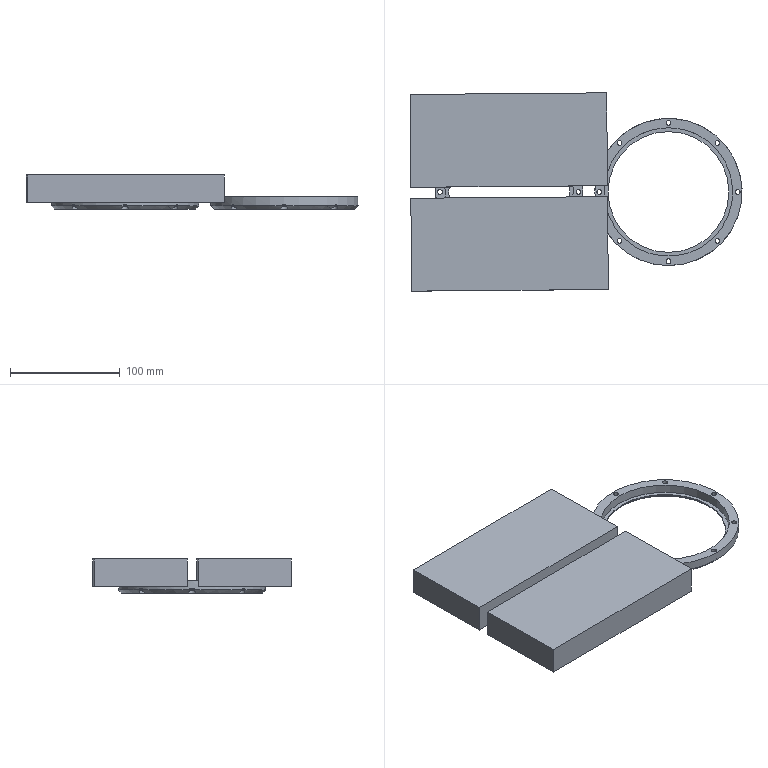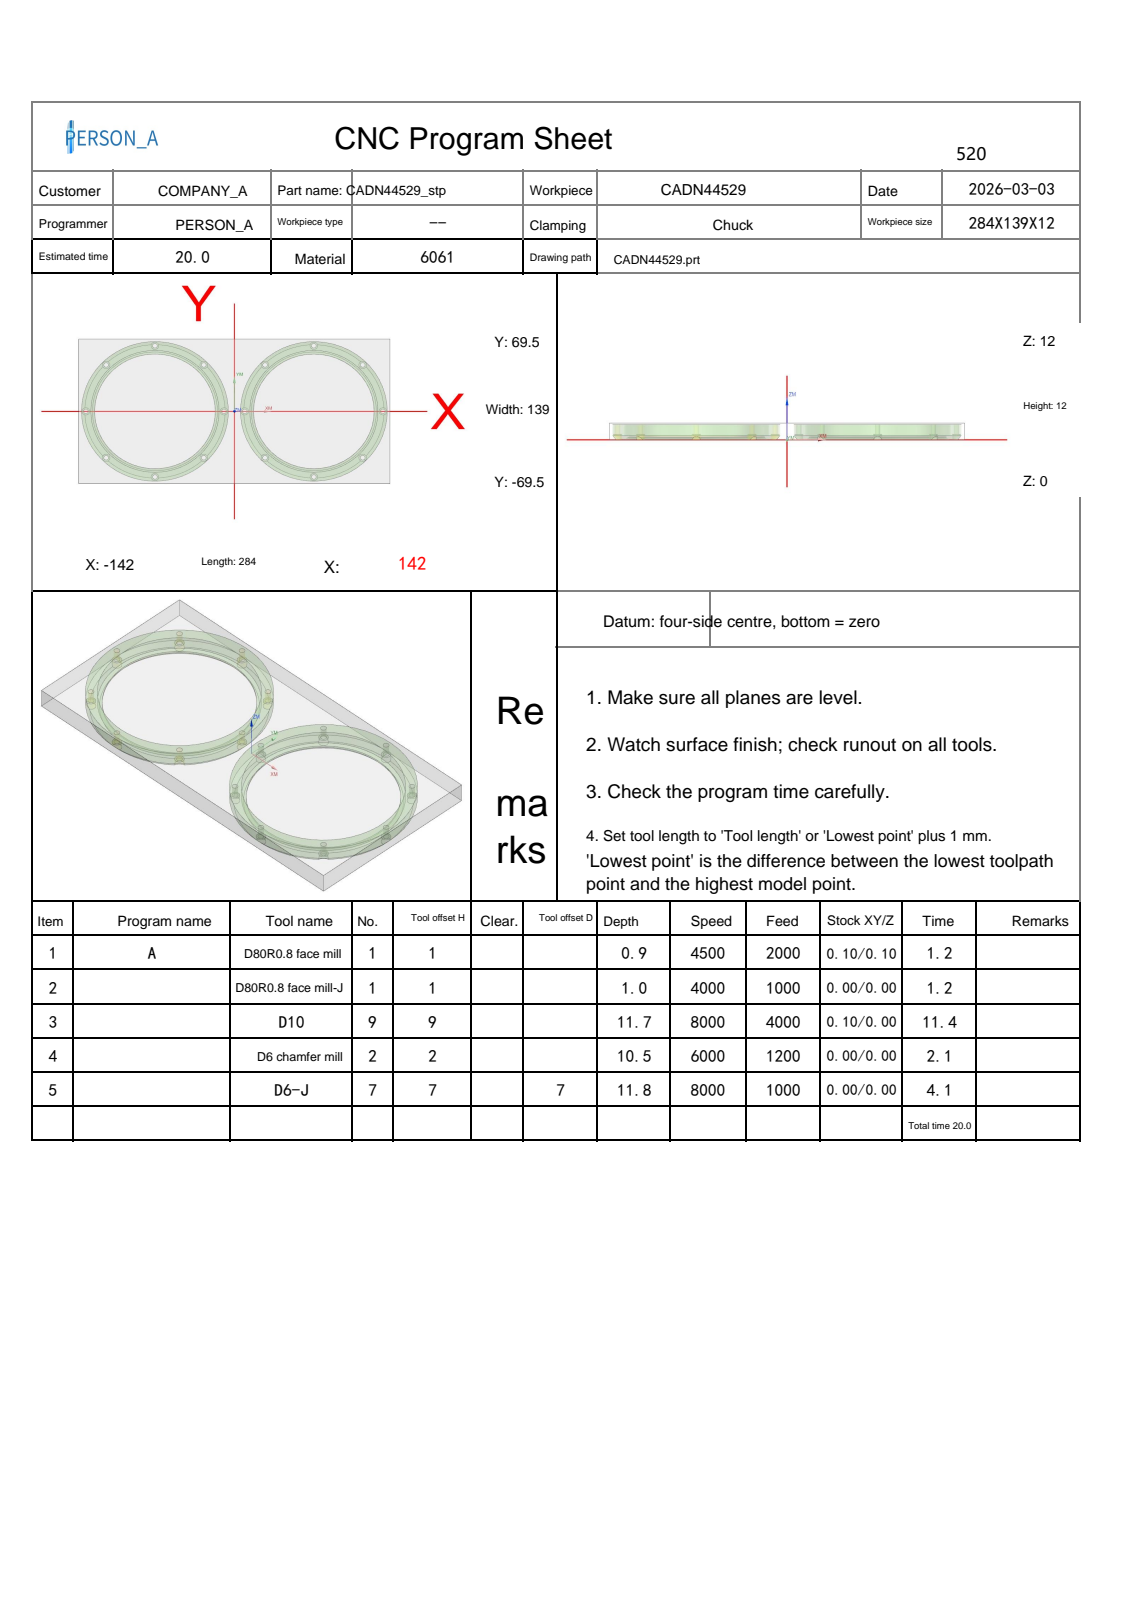NC program | NX | posted by the shop | part box 302.234 x 180.468 x 31 mm
Whole program:
%
O0001
(Machine time: 20.83 MIN)
(===Total Tool:4===)
(T1=D80R0.8 face mill D=80.  R=0.8  D-  H01 Z=11.   )
(T9=D10     D=10.  R=0.   D-  H09 Z=0.3   )
(T2=D6 chamfer mill   D=6.   R=0.   D-  H02 Z=1.5   )
(T7=D6-J    D=6.   R=0.   D7  H07 Z=0.2   )
G80 G90 G17 G49 G40
G91 G28 Z0
M01
N1 T01 M06
(D80R0.8 face mill  D=80. R=0.8 H=01 ce=0.10 di=0.10)
G00 G90 G54 X-183.526 Y43.097 M03 S4500
G43 H01 Z61.
M08
Z13.55
G01 Z11.55 F2000.
X-170.543
X165.174
G02 X172.655 Y37.93 I0.0 J-8.
X178.96 Y11.664 I-100.155 J-37.93
X179.003 Y10.88 I-7.157 J-.784
X171.803 Y3.68 I-7.2 J0.0
G01 X-172.338
G03 X-179.535 Y-3.52 I.004 J-7.2
X-179.531 Y-3.77 I7.2 J0.0
X-175.316 Y-29.976 I107.031 J3.77
X-167.636 Y-35.737 I7.68 J2.239
G01 X173.459
X186.109
Z13.55
G00 X-183.526 Y43.097
Z13.1
G01 Z11.1
X-170.543
X165.174
G02 X172.655 Y37.93 I0.0 J-8.
X178.96 Y11.664 I-100.155 J-37.93
X179.003 Y10.88 I-7.157 J-.784
X171.803 Y3.68 I-7.2 J0.0
G01 X-172.338
G03 X-179.535 Y-3.52 I.004 J-7.2
X-179.531 Y-3.77 I7.2 J0.0
X-175.316 Y-29.976 I107.031 J3.77
X-167.636 Y-35.737 I7.68 J2.239
G01 X173.459
X186.109
Z13.1
G00 Z61.
G91 G28 Z0.0
M05
M09
G91 G28 Z0.0
M01
N2 T01 M06
(D80R0.8 face mill-J  D=80. R=0.8 H=01 ce=0.00 di=0.00)
G00 G90 G54 X-183.459 Y42.999 M03 S4000
G43 H01 Z61.
M08
Z13.
G01 Z11. F1000.
X-170.479
X165.106
G02 X172.589 Y37.827 I0.0 J-8.
X178.861 Y11.665 I-100.089 J-37.827
X178.904 Y10.88 I-7.157 J-.785
X171.704 Y3.68 I-7.2 J0.0
G01 X-172.24
G03 X-179.437 Y-3.52 I.004 J-7.2
X-179.433 Y-3.77 I7.2 J0.0
X-175.244 Y-29.872 I106.933 J3.77
X-167.563 Y-35.639 I7.682 J2.233
G01 X173.389
X186.037
Z13.
G00 Z61.
G91 G28 Z0.0
M05
M09
G91 G28 Z0.0
M01
N3 T09 M06
(D10  D=10. R=0. H=09 ce=0.10 di=0.10)
G00 G90 G54 X-118.783 Y18.61 M03 S8000
G43 H09 Z61.
M08
Z13.
G01 X-119.955 Y15.526 Z12.827 F4000.
X-121.201 Y11.011 Z12.581
X-122.018 Y6.399 Z12.336
X-122.4 Y1.731 Z12.09
Y0.0 Z12.
G03 X-72.5 Y-49.9 Z11.854 I49.9 J0.0
X-22.6 Y0.0 Z11.707 I0.0 J49.9
X-72.5 Y49.9 Z11.561 I-49.9 J0.0
X-122.4 Y0.0 Z11.415 I0.0 J-49.9
X-72.5 Y-49.9 Z11.269 I49.9 J0.0
X-22.6 Y0.0 Z11.122 I0.0 J49.9
X-72.5 Y49.9 Z10.976 I-49.9 J0.0
X-122.4 Y0.0 Z10.83 I0.0 J-49.9
X-72.5 Y-49.9 Z10.684 I49.9 J0.0
X-22.6 Y0.0 Z10.537 I0.0 J49.9
X-72.5 Y49.9 Z10.391 I-49.9 J0.0
X-122.4 Y0.0 Z10.245 I0.0 J-49.9
X-72.5 Y-49.9 Z10.099 I49.9 J0.0
X-22.6 Y0.0 Z9.952 I0.0 J49.9
X-72.5 Y49.9 Z9.806 I-49.9 J0.0
X-122.4 Y0.0 Z9.66 I0.0 J-49.9
X-72.5 Y-49.9 Z9.514 I49.9 J0.0
X-22.6 Y0.0 Z9.367 I0.0 J49.9
X-72.5 Y49.9 Z9.221 I-49.9 J0.0
X-122.4 Y0.0 Z9.075 I0.0 J-49.9
X-72.5 Y-49.9 Z8.929 I49.9 J0.0
X-22.6 Y0.0 Z8.782 I0.0 J49.9
X-72.5 Y49.9 Z8.636 I-49.9 J0.0
X-122.4 Y0.0 Z8.49 I0.0 J-49.9
X-72.5 Y-49.9 Z8.344 I49.9 J0.0
X-22.6 Y0.0 Z8.197 I0.0 J49.9
X-72.5 Y49.9 Z8.051 I-49.9 J0.0
X-122.4 Y0.0 Z7.905 I0.0 J-49.9
X-72.5 Y-49.9 Z7.759 I49.9 J0.0
X-22.6 Y0.0 Z7.612 I0.0 J49.9
X-72.5 Y49.9 Z7.466 I-49.9 J0.0
X-122.4 Y0.0 Z7.32 I0.0 J-49.9
X-72.5 Y-49.9 Z7.174 I49.9 J0.0
X-22.6 Y0.0 Z7.027 I0.0 J49.9
X-72.5 Y49.9 Z6.881 I-49.9 J0.0
X-122.4 Y0.0 Z6.735 I0.0 J-49.9
X-72.5 Y-49.9 Z6.589 I49.9 J0.0
X-22.6 Y0.0 Z6.442 I0.0 J49.9
X-72.5 Y49.9 Z6.296 I-49.9 J0.0
X-122.4 Y0.0 Z6.15 I0.0 J-49.9
X-72.5 Y-49.9 Z6.004 I49.9 J0.0
X-22.6 Y0.0 Z5.857 I0.0 J49.9
X-72.5 Y49.9 Z5.711 I-49.9 J0.0
X-122.4 Y0.0 Z5.565 I0.0 J-49.9
X-72.5 Y-49.9 Z5.419 I49.9 J0.0
X-22.6 Y0.0 Z5.272 I0.0 J49.9
X-72.5 Y49.9 Z5.126 I-49.9 J0.0
X-122.4 Y0.0 Z4.98 I0.0 J-49.9
X-72.5 Y-49.9 Z4.834 I49.9 J0.0
X-22.6 Y0.0 Z4.687 I0.0 J49.9
X-72.5 Y49.9 Z4.541 I-49.9 J0.0
X-122.4 Y0.0 Z4.395 I0.0 J-49.9
X-72.5 Y-49.9 Z4.249 I49.9 J0.0
X-22.6 Y0.0 Z4.103 I0.0 J49.9
X-72.5 Y49.9 Z3.956 I-49.9 J0.0
X-122.4 Y0.0 Z3.81 I0.0 J-49.9
X-72.5 Y-49.9 Z3.664 I49.9 J0.0
X-22.6 Y0.0 Z3.518 I0.0 J49.9
X-72.5 Y49.9 Z3.371 I-49.9 J0.0
X-122.4 Y0.0 Z3.225 I0.0 J-49.9
X-72.5 Y-49.9 Z3.079 I49.9 J0.0
X-22.6 Y0.0 Z2.933 I0.0 J49.9
X-72.5 Y49.9 Z2.786 I-49.9 J0.0
X-122.4 Y0.0 Z2.64 I0.0 J-49.9
X-72.5 Y-49.9 Z2.494 I49.9 J0.0
X-22.6 Y0.0 Z2.348 I0.0 J49.9
X-72.5 Y49.9 Z2.201 I-49.9 J0.0
X-122.4 Y0.0 Z2.055 I0.0 J-49.9
X-72.5 Y-49.9 Z1.909 I49.9 J0.0
X-22.6 Y0.0 Z1.763 I0.0 J49.9
X-72.5 Y49.9 Z1.616 I-49.9 J0.0
X-122.4 Y0.0 Z1.47 I0.0 J-49.9
X-72.5 Y-49.9 Z1.324 I49.9 J0.0
X-22.6 Y0.0 Z1.178 I0.0 J49.9
X-72.5 Y49.9 Z1.031 I-49.9 J0.0
X-122.4 Y0.0 Z.885 I0.0 J-49.9
X-72.5 Y-49.9 Z.739 I49.9 J0.0
X-22.6 Y0.0 Z.593 I0.0 J49.9
X-72.5 Y49.9 Z.446 I-49.9 J0.0
X-122.4 Y0.0 Z.3 I0.0 J-49.9
X-72.5 Y-49.9 I49.9 J0.0
X-22.6 Y0.0 I0.0 J49.9
X-72.5 Y49.9 I-49.9 J0.0
X-122.4 Y0.0 I0.0 J-49.9
X-122.398 Y-.4 I49.9 J0.0
G01 Z1.3
G00 Z61.
X53.89 Y-46.283
Z13.
G01 X56.974 Y-47.455 Z12.827
X61.489 Y-48.701 Z12.581
X66.101 Y-49.518 Z12.336
X70.769 Y-49.9 Z12.09
X72.5 Z12.
G03 X122.4 Y0.0 Z11.854 I0.0 J49.9
X72.5 Y49.9 Z11.707 I-49.9 J0.0
X22.6 Y0.0 Z11.561 I0.0 J-49.9
X72.5 Y-49.9 Z11.415 I49.9 J0.0
X122.4 Y0.0 Z11.269 I0.0 J49.9
X72.5 Y49.9 Z11.122 I-49.9 J0.0
X22.6 Y0.0 Z10.976 I0.0 J-49.9
X72.5 Y-49.9 Z10.83 I49.9 J0.0
X122.4 Y0.0 Z10.684 I0.0 J49.9
X72.5 Y49.9 Z10.537 I-49.9 J0.0
X22.6 Y0.0 Z10.391 I0.0 J-49.9
X72.5 Y-49.9 Z10.245 I49.9 J0.0
X122.4 Y0.0 Z10.099 I0.0 J49.9
X72.5 Y49.9 Z9.952 I-49.9 J0.0
X22.6 Y0.0 Z9.806 I0.0 J-49.9
X72.5 Y-49.9 Z9.66 I49.9 J0.0
X122.4 Y0.0 Z9.514 I0.0 J49.9
X72.5 Y49.9 Z9.367 I-49.9 J0.0
X22.6 Y0.0 Z9.221 I0.0 J-49.9
X72.5 Y-49.9 Z9.075 I49.9 J0.0
X122.4 Y0.0 Z8.929 I0.0 J49.9
X72.5 Y49.9 Z8.782 I-49.9 J0.0
X22.6 Y0.0 Z8.636 I0.0 J-49.9
X72.5 Y-49.9 Z8.49 I49.9 J0.0
X122.4 Y0.0 Z8.344 I0.0 J49.9
X72.5 Y49.9 Z8.197 I-49.9 J0.0
X22.6 Y0.0 Z8.051 I0.0 J-49.9
X72.5 Y-49.9 Z7.905 I49.9 J0.0
X122.4 Y0.0 Z7.759 I0.0 J49.9
X72.5 Y49.9 Z7.612 I-49.9 J0.0
X22.6 Y0.0 Z7.466 I0.0 J-49.9
X72.5 Y-49.9 Z7.32 I49.9 J0.0
X122.4 Y0.0 Z7.174 I0.0 J49.9
X72.5 Y49.9 Z7.027 I-49.9 J0.0
X22.6 Y0.0 Z6.881 I0.0 J-49.9
X72.5 Y-49.9 Z6.735 I49.9 J0.0
X122.4 Y0.0 Z6.589 I0.0 J49.9
X72.5 Y49.9 Z6.442 I-49.9 J0.0
X22.6 Y0.0 Z6.296 I0.0 J-49.9
X72.5 Y-49.9 Z6.15 I49.9 J0.0
X122.4 Y0.0 Z6.004 I0.0 J49.9
X72.5 Y49.9 Z5.857 I-49.9 J0.0
X22.6 Y0.0 Z5.711 I0.0 J-49.9
X72.5 Y-49.9 Z5.565 I49.9 J0.0
X122.4 Y0.0 Z5.419 I0.0 J49.9
X72.5 Y49.9 Z5.272 I-49.9 J0.0
X22.6 Y0.0 Z5.126 I0.0 J-49.9
X72.5 Y-49.9 Z4.98 I49.9 J0.0
X122.4 Y0.0 Z4.834 I0.0 J49.9
X72.5 Y49.9 Z4.687 I-49.9 J0.0
X22.6 Y0.0 Z4.541 I0.0 J-49.9
X72.5 Y-49.9 Z4.395 I49.9 J0.0
X122.4 Y0.0 Z4.249 I0.0 J49.9
X72.5 Y49.9 Z4.103 I-49.9 J0.0
X22.6 Y0.0 Z3.956 I0.0 J-49.9
X72.5 Y-49.9 Z3.81 I49.9 J0.0
X122.4 Y0.0 Z3.664 I0.0 J49.9
X72.5 Y49.9 Z3.518 I-49.9 J0.0
X22.6 Y0.0 Z3.371 I0.0 J-49.9
X72.5 Y-49.9 Z3.225 I49.9 J0.0
X122.4 Y0.0 Z3.079 I0.0 J49.9
X72.5 Y49.9 Z2.933 I-49.9 J0.0
X22.6 Y0.0 Z2.786 I0.0 J-49.9
X72.5 Y-49.9 Z2.64 I49.9 J0.0
X122.4 Y0.0 Z2.494 I0.0 J49.9
X72.5 Y49.9 Z2.348 I-49.9 J0.0
X22.6 Y0.0 Z2.201 I0.0 J-49.9
X72.5 Y-49.9 Z2.055 I49.9 J0.0
X122.4 Y0.0 Z1.909 I0.0 J49.9
X72.5 Y49.9 Z1.763 I-49.9 J0.0
X22.6 Y0.0 Z1.616 I0.0 J-49.9
X72.5 Y-49.9 Z1.47 I49.9 J0.0
X122.4 Y0.0 Z1.324 I0.0 J49.9
X72.5 Y49.9 Z1.178 I-49.9 J0.0
X22.6 Y0.0 Z1.031 I0.0 J-49.9
X72.5 Y-49.9 Z.885 I49.9 J0.0
X122.4 Y0.0 Z.739 I0.0 J49.9
X72.5 Y49.9 Z.593 I-49.9 J0.0
X22.6 Y0.0 Z.446 I0.0 J-49.9
X72.5 Y-49.9 Z.3 I49.9 J0.0
X122.4 Y0.0 I0.0 J49.9
X72.5 Y49.9 I-49.9 J0.0
X22.6 Y0.0 I0.0 J-49.9
X72.5 Y-49.9 I49.9 J0.0
X72.9 Y-49.898 I0.0 J49.9
G01 Z1.3
G00 Z61.
G00 G90 X-91.164 Y-50.002 M03 S8000
Z61.
Z12.
G01 X-89.077 Y-50.793 Z11.883 F4000.
X-84.237 Y-52.125 Z11.62
X-79.294 Y-52.996 Z11.357
X-74.29 Y-53.4 Z11.094
X-72.5 Z11.
G03 X-19.1 Y0.0 Z10.859 I0.0 J53.4
X-72.5 Y53.4 Z10.718 I-53.4 J0.0
X-125.9 Y0.0 Z10.577 I0.0 J-53.4
X-72.5 Y-53.4 Z10.436 I53.4 J0.0
X-19.1 Y0.0 Z10.295 I0.0 J53.4
X-72.5 Y53.4 Z10.154 I-53.4 J0.0
X-125.9 Y0.0 Z10.013 I0.0 J-53.4
X-72.5 Y-53.4 Z9.872 I53.4 J0.0
X-19.1 Y0.0 Z9.73 I0.0 J53.4
X-72.5 Y53.4 Z9.589 I-53.4 J0.0
X-125.9 Y0.0 Z9.448 I0.0 J-53.4
X-72.5 Y-53.4 Z9.307 I53.4 J0.0
X-19.1 Y0.0 Z9.166 I0.0 J53.4
X-72.5 Y53.4 Z9.025 I-53.4 J0.0
X-125.9 Y0.0 Z8.884 I0.0 J-53.4
X-72.5 Y-53.4 Z8.743 I53.4 J0.0
X-19.1 Y0.0 Z8.602 I0.0 J53.4
X-72.5 Y53.4 Z8.461 I-53.4 J0.0
X-125.9 Y0.0 Z8.32 I0.0 J-53.4
X-72.5 Y-53.4 Z8.179 I53.4 J0.0
X-19.1 Y0.0 Z8.038 I0.0 J53.4
X-72.5 Y53.4 Z7.897 I-53.4 J0.0
X-125.9 Y0.0 Z7.755 I0.0 J-53.4
X-72.5 Y-53.4 Z7.614 I53.4 J0.0
X-19.1 Y0.0 Z7.473 I0.0 J53.4
X-72.5 Y53.4 Z7.332 I-53.4 J0.0
X-125.9 Y0.0 Z7.191 I0.0 J-53.4
X-72.5 Y-53.4 Z7.05 I53.4 J0.0
X-19.1 Y0.0 Z6.909 I0.0 J53.4
X-72.5 Y53.4 Z6.768 I-53.4 J0.0
X-125.9 Y0.0 Z6.627 I0.0 J-53.4
X-72.5 Y-53.4 Z6.486 I53.4 J0.0
X-19.1 Y0.0 Z6.345 I0.0 J53.4
X-72.5 Y53.4 Z6.204 I-53.4 J0.0
X-125.9 Y0.0 Z6.063 I0.0 J-53.4
X-72.5 Y-53.4 Z5.922 I53.4 J0.0
X-19.1 Y0.0 Z5.78 I0.0 J53.4
X-72.5 Y53.4 Z5.639 I-53.4 J0.0
X-125.9 Y0.0 Z5.498 I0.0 J-53.4
X-72.5 Y-53.4 Z5.357 I53.4 J0.0
X-19.1 Y0.0 Z5.216 I0.0 J53.4
X-72.5 Y53.4 Z5.075 I-53.4 J0.0
X-125.9 Y0.0 Z4.934 I0.0 J-53.4
X-72.5 Y-53.4 Z4.793 I53.4 J0.0
X-19.1 Y0.0 Z4.652 I0.0 J53.4
X-72.5 Y53.4 Z4.511 I-53.4 J0.0
X-125.9 Y0.0 Z4.37 I0.0 J-53.4
X-72.5 Y-53.4 Z4.229 I53.4 J0.0
X-19.1 Y0.0 Z4.088 I0.0 J53.4
X-72.5 Y53.4 Z3.947 I-53.4 J0.0
X-125.9 Y0.0 Z3.805 I0.0 J-53.4
X-72.5 Y-53.4 Z3.664 I53.4 J0.0
X-19.1 Y0.0 Z3.523 I0.0 J53.4
X-72.5 Y53.4 Z3.382 I-53.4 J0.0
X-125.9 Y0.0 Z3.241 I0.0 J-53.4
X-72.5 Y-53.4 Z3.1 I53.4 J0.0
X-19.1 Y0.0 I0.0 J53.4
X-72.5 Y53.4 I-53.4 J0.0
X-125.9 Y0.0 I0.0 J-53.4
X-72.5 Y-53.4 I53.4 J0.0
X-72.1 Y-53.399 I0.0 J53.4
G01 Z4.1
G00 Z61.
X53.836 Y-50.002
Z12.
G01 X55.923 Y-50.793 Z11.883
X60.763 Y-52.125 Z11.62
X65.706 Y-52.996 Z11.357
X70.71 Y-53.4 Z11.094
X72.5 Z11.
G03 X125.9 Y0.0 Z10.859 I0.0 J53.4
X72.5 Y53.4 Z10.718 I-53.4 J0.0
X19.1 Y0.0 Z10.577 I0.0 J-53.4
X72.5 Y-53.4 Z10.436 I53.4 J0.0
X125.9 Y0.0 Z10.295 I0.0 J53.4
X72.5 Y53.4 Z10.154 I-53.4 J0.0
X19.1 Y0.0 Z10.013 I0.0 J-53.4
X72.5 Y-53.4 Z9.872 I53.4 J0.0
X125.9 Y0.0 Z9.73 I0.0 J53.4
X72.5 Y53.4 Z9.589 I-53.4 J0.0
X19.1 Y0.0 Z9.448 I0.0 J-53.4
X72.5 Y-53.4 Z9.307 I53.4 J0.0
X125.9 Y0.0 Z9.166 I0.0 J53.4
X72.5 Y53.4 Z9.025 I-53.4 J0.0
X19.1 Y0.0 Z8.884 I0.0 J-53.4
X72.5 Y-53.4 Z8.743 I53.4 J0.0
X125.9 Y0.0 Z8.602 I0.0 J53.4
X72.5 Y53.4 Z8.461 I-53.4 J0.0
X19.1 Y0.0 Z8.32 I0.0 J-53.4
X72.5 Y-53.4 Z8.179 I53.4 J0.0
X125.9 Y0.0 Z8.038 I0.0 J53.4
X72.5 Y53.4 Z7.897 I-53.4 J0.0
X19.1 Y0.0 Z7.755 I0.0 J-53.4
X72.5 Y-53.4 Z7.614 I53.4 J0.0
X125.9 Y0.0 Z7.473 I0.0 J53.4
X72.5 Y53.4 Z7.332 I-53.4 J0.0
X19.1 Y0.0 Z7.191 I0.0 J-53.4
X72.5 Y-53.4 Z7.05 I53.4 J0.0
X125.9 Y0.0 Z6.909 I0.0 J53.4
X72.5 Y53.4 Z6.768 I-53.4 J0.0
X19.1 Y0.0 Z6.627 I0.0 J-53.4
X72.5 Y-53.4 Z6.486 I53.4 J0.0
X125.9 Y0.0 Z6.345 I0.0 J53.4
X72.5 Y53.4 Z6.204 I-53.4 J0.0
X19.1 Y0.0 Z6.063 I0.0 J-53.4
X72.5 Y-53.4 Z5.922 I53.4 J0.0
X125.9 Y0.0 Z5.78 I0.0 J53.4
X72.5 Y53.4 Z5.639 I-53.4 J0.0
X19.1 Y0.0 Z5.498 I0.0 J-53.4
X72.5 Y-53.4 Z5.357 I53.4 J0.0
X125.9 Y0.0 Z5.216 I0.0 J53.4
X72.5 Y53.4 Z5.075 I-53.4 J0.0
X19.1 Y0.0 Z4.934 I0.0 J-53.4
X72.5 Y-53.4 Z4.793 I53.4 J0.0
X125.9 Y0.0 Z4.652 I0.0 J53.4
X72.5 Y53.4 Z4.511 I-53.4 J0.0
X19.1 Y0.0 Z4.37 I0.0 J-53.4
X72.5 Y-53.4 Z4.229 I53.4 J0.0
X125.9 Y0.0 Z4.088 I0.0 J53.4
X72.5 Y53.4 Z3.947 I-53.4 J0.0
X19.1 Y0.0 Z3.805 I0.0 J-53.4
X72.5 Y-53.4 Z3.664 I53.4 J0.0
X125.9 Y0.0 Z3.523 I0.0 J53.4
X72.5 Y53.4 Z3.382 I-53.4 J0.0
X19.1 Y0.0 Z3.241 I0.0 J-53.4
X72.5 Y-53.4 Z3.1 I53.4 J0.0
X125.9 Y0.0 I0.0 J53.4
X72.5 Y53.4 I-53.4 J0.0
X19.1 Y0.0 I0.0 J-53.4
X72.5 Y-53.4 I53.4 J0.0
X72.9 Y-53.399 I0.0 J53.4
G01 Z4.1
G00 Z61.
G00 G90 X72.5 Y-72.1 M03 S6000
Z61.
Z11.5
G02 X.4 Y0.0 Z11.381 I0.0 J72.1 F4000.
X72.5 Y72.1 Z11.261 I72.1 J0.0
X144.6 Y0.0 Z11.141 I0.0 J-72.1
X72.5 Y-72.1 Z11.022 I-72.1 J0.0
X.4 Y0.0 Z10.902 I0.0 J72.1
X72.5 Y72.1 Z10.783 I72.1 J0.0
X144.6 Y0.0 Z10.663 I0.0 J-72.1
X72.5 Y-72.1 Z10.544 I-72.1 J0.0
X.4 Y0.0 Z10.424 I0.0 J72.1
X72.5 Y72.1 Z10.304 I72.1 J0.0
X144.6 Y0.0 Z10.185 I0.0 J-72.1
X72.5 Y-72.1 Z10.065 I-72.1 J0.0
X.4 Y0.0 Z9.946 I0.0 J72.1
X72.5 Y72.1 Z9.826 I72.1 J0.0
X144.6 Y0.0 Z9.707 I0.0 J-72.1
X72.5 Y-72.1 Z9.587 I-72.1 J0.0
X.4 Y0.0 Z9.467 I0.0 J72.1
X72.5 Y72.1 Z9.348 I72.1 J0.0
X144.6 Y0.0 Z9.228 I0.0 J-72.1
X72.5 Y-72.1 Z9.109 I-72.1 J0.0
X.4 Y0.0 Z8.989 I0.0 J72.1
X72.5 Y72.1 Z8.87 I72.1 J0.0
X144.6 Y0.0 Z8.75 I0.0 J-72.1
X72.5 Y-72.1 Z8.631 I-72.1 J0.0
X.4 Y0.0 Z8.511 I0.0 J72.1
X72.5 Y72.1 Z8.391 I72.1 J0.0
X144.6 Y0.0 Z8.272 I0.0 J-72.1
X72.5 Y-72.1 Z8.152 I-72.1 J0.0
X.4 Y0.0 Z8.033 I0.0 J72.1
X72.5 Y72.1 Z7.913 I72.1 J0.0
X144.6 Y0.0 Z7.794 I0.0 J-72.1
X72.5 Y-72.1 Z7.674 I-72.1 J0.0
X.4 Y0.0 Z7.554 I0.0 J72.1
X72.5 Y72.1 Z7.435 I72.1 J0.0
X144.6 Y0.0 Z7.315 I0.0 J-72.1
X72.5 Y-72.1 Z7.196 I-72.1 J0.0
X.4 Y0.0 Z7.076 I0.0 J72.1
X72.5 Y72.1 Z6.957 I72.1 J0.0
X144.6 Y0.0 Z6.837 I0.0 J-72.1
X72.5 Y-72.1 Z6.717 I-72.1 J0.0
X.4 Y0.0 Z6.598 I0.0 J72.1
X72.5 Y72.1 Z6.478 I72.1 J0.0
X144.6 Y0.0 Z6.359 I0.0 J-72.1
X72.5 Y-72.1 Z6.239 I-72.1 J0.0
X.4 Y0.0 Z6.12 I0.0 J72.1
X72.5 Y72.1 Z6. I72.1 J0.0
X144.6 Y0.0 Z5.88 I0.0 J-72.1
X72.5 Y-72.1 Z5.761 I-72.1 J0.0
X.4 Y0.0 Z5.641 I0.0 J72.1
X72.5 Y72.1 Z5.522 I72.1 J0.0
X144.6 Y0.0 Z5.402 I0.0 J-72.1
X72.5 Y-72.1 Z5.283 I-72.1 J0.0
X.4 Y0.0 Z5.163 I0.0 J72.1
X72.5 Y72.1 Z5.044 I72.1 J0.0
X144.6 Y0.0 Z4.924 I0.0 J-72.1
X72.5 Y-72.1 Z4.804 I-72.1 J0.0
X.4 Y0.0 Z4.685 I0.0 J72.1
X72.5 Y72.1 Z4.565 I72.1 J0.0
X144.6 Y0.0 Z4.446 I0.0 J-72.1
X72.5 Y-72.1 Z4.326 I-72.1 J0.0
X.4 Y0.0 Z4.207 I0.0 J72.1
X72.5 Y72.1 Z4.087 I72.1 J0.0
X144.6 Y0.0 Z3.967 I0.0 J-72.1
X72.5 Y-72.1 Z3.848 I-72.1 J0.0
X.4 Y0.0 Z3.728 I0.0 J72.1
X72.5 Y72.1 Z3.609 I72.1 J0.0
X144.6 Y0.0 Z3.489 I0.0 J-72.1
X72.5 Y-72.1 Z3.37 I-72.1 J0.0
X.4 Y0.0 Z3.25 I0.0 J72.1
X72.5 Y72.1 Z3.13 I72.1 J0.0
X144.6 Y0.0 Z3.011 I0.0 J-72.1
X72.5 Y-72.1 Z2.891 I-72.1 J0.0
X.4 Y0.0 Z2.772 I0.0 J72.1
X72.5 Y72.1 Z2.652 I72.1 J0.0
X144.6 Y0.0 Z2.533 I0.0 J-72.1
X72.5 Y-72.1 Z2.413 I-72.1 J0.0
X.4 Y0.0 Z2.293 I0.0 J72.1
X72.5 Y72.1 Z2.174 I72.1 J0.0
X144.6 Y0.0 Z2.054 I0.0 J-72.1
X72.5 Y-72.1 Z1.935 I-72.1 J0.0
X.4 Y0.0 Z1.815 I0.0 J72.1
X72.5 Y72.1 Z1.696 I72.1 J0.0
X144.6 Y0.0 Z1.576 I0.0 J-72.1
X72.5 Y-72.1 Z1.457 I-72.1 J0.0
X.4 Y0.0 Z1.337 I0.0 J72.1
X72.5 Y72.1 Z1.217 I72.1 J0.0
X144.6 Y0.0 Z1.098 I0.0 J-72.1
X72.5 Y-72.1 Z.978 I-72.1 J0.0
X.4 Y0.0 Z.859 I0.0 J72.1
X72.5 Y72.1 Z.739 I72.1 J0.0
X144.6 Y0.0 Z.62 I0.0 J-72.1
X72.5 Y-72.1 Z.5 I-72.1 J0.0
X.4 Y0.0 I0.0 J72.1
X72.5 Y72.1 I72.1 J0.0
X144.6 Y0.0 I0.0 J-72.1
X72.5 Y-72.1 I-72.1 J0.0
X72. Y-72.098 I0.0 J72.1
G01 Z1.5
G00 Z61.
X-72.5 Y-72.1
Z11.5
G02 X-144.6 Y0.0 Z11.381 I0.0 J72.1
X-72.5 Y72.1 Z11.261 I72.1 J0.0
X-.4 Y0.0 Z11.141 I0.0 J-72.1
X-72.5 Y-72.1 Z11.022 I-72.1 J0.0
X-144.6 Y0.0 Z10.902 I0.0 J72.1
X-72.5 Y72.1 Z10.783 I72.1 J0.0
X-.4 Y0.0 Z10.663 I0.0 J-72.1
X-72.5 Y-72.1 Z10.544 I-72.1 J0.0
X-144.6 Y0.0 Z10.424 I0.0 J72.1
X-72.5 Y72.1 Z10.304 I72.1 J0.0
X-.4 Y0.0 Z10.185 I0.0 J-72.1
X-72.5 Y-72.1 Z10.065 I-72.1 J0.0
X-144.6 Y0.0 Z9.946 I0.0 J72.1
X-72.5 Y72.1 Z9.826 I72.1 J0.0
X-.4 Y0.0 Z9.707 I0.0 J-72.1
X-72.5 Y-72.1 Z9.587 I-72.1 J0.0
X-144.6 Y0.0 Z9.467 I0.0 J72.1
X-72.5 Y72.1 Z9.348 I72.1 J0.0
X-.4 Y0.0 Z9.228 I0.0 J-72.1
X-72.5 Y-72.1 Z9.109 I-72.1 J0.0
X-144.6 Y0.0 Z8.989 I0.0 J72.1
X-72.5 Y72.1 Z8.87 I72.1 J0.0
X-.4 Y0.0 Z8.75 I0.0 J-72.1
X-72.5 Y-72.1 Z8.631 I-72.1 J0.0
X-144.6 Y0.0 Z8.511 I0.0 J72.1
X-72.5 Y72.1 Z8.391 I72.1 J0.0
X-.4 Y0.0 Z8.272 I0.0 J-72.1
X-72.5 Y-72.1 Z8.152 I-72.1 J0.0
X-144.6 Y0.0 Z8.033 I0.0 J72.1
X-72.5 Y72.1 Z7.913 I72.1 J0.0
X-.4 Y0.0 Z7.794 I0.0 J-72.1
X-72.5 Y-72.1 Z7.674 I-72.1 J0.0
X-144.6 Y0.0 Z7.554 I0.0 J72.1
X-72.5 Y72.1 Z7.435 I72.1 J0.0
X-.4 Y0.0 Z7.315 I0.0 J-72.1
X-72.5 Y-72.1 Z7.196 I-72.1 J0.0
X-144.6 Y0.0 Z7.076 I0.0 J72.1
X-72.5 Y72.1 Z6.957 I72.1 J0.0
X-.4 Y0.0 Z6.837 I0.0 J-72.1
X-72.5 Y-72.1 Z6.717 I-72.1 J0.0
X-144.6 Y0.0 Z6.598 I0.0 J72.1
X-72.5 Y72.1 Z6.478 I72.1 J0.0
X-.4 Y0.0 Z6.359 I0.0 J-72.1
X-72.5 Y-72.1 Z6.239 I-72.1 J0.0
X-144.6 Y0.0 Z6.12 I0.0 J72.1
X-72.5 Y72.1 Z6. I72.1 J0.0
X-.4 Y0.0 Z5.88 I0.0 J-72.1
X-72.5 Y-72.1 Z5.761 I-72.1 J0.0
X-144.6 Y0.0 Z5.641 I0.0 J72.1
X-72.5 Y72.1 Z5.522 I72.1 J0.0
X-.4 Y0.0 Z5.402 I0.0 J-72.1
X-72.5 Y-72.1 Z5.283 I-72.1 J0.0
X-144.6 Y0.0 Z5.163 I0.0 J72.1
X-72.5 Y72.1 Z5.044 I72.1 J0.0
X-.4 Y0.0 Z4.924 I0.0 J-72.1
X-72.5 Y-72.1 Z4.804 I-72.1 J0.0
X-144.6 Y0.0 Z4.685 I0.0 J72.1
X-72.5 Y72.1 Z4.565 I72.1 J0.0
X-.4 Y0.0 Z4.446 I0.0 J-72.1
X-72.5 Y-72.1 Z4.326 I-72.1 J0.0
X-144.6 Y0.0 Z4.207 I0.0 J72.1
X-72.5 Y72.1 Z4.087 I72.1 J0.0
X-.4 Y0.0 Z3.967 I0.0 J-72.1
X-72.5 Y-72.1 Z3.848 I-72.1 J0.0
X-144.6 Y0.0 Z3.728 I0.0 J72.1
X-72.5 Y72.1 Z3.609 I72.1 J0.0
X-.4 Y0.0 Z3.489 I0.0 J-72.1
X-72.5 Y-72.1 Z3.37 I-72.1 J0.0
X-144.6 Y0.0 Z3.25 I0.0 J72.1
X-72.5 Y72.1 Z3.13 I72.1 J0.0
X-.4 Y0.0 Z3.011 I0.0 J-72.1
X-72.5 Y-72.1 Z2.891 I-72.1 J0.0
X-144.6 Y0.0 Z2.772 I0.0 J72.1
X-72.5 Y72.1 Z2.652 I72.1 J0.0
X-.4 Y0.0 Z2.533 I0.0 J-72.1
X-72.5 Y-72.1 Z2.413 I-72.1 J0.0
X-144.6 Y0.0 Z2.293 I0.0 J72.1
X-72.5 Y72.1 Z2.174 I72.1 J0.0
X-.4 Y0.0 Z2.054 I0.0 J-72.1
X-72.5 Y-72.1 Z1.935 I-72.1 J0.0
X-144.6 Y0.0 Z1.815 I0.0 J72.1
X-72.5 Y72.1 Z1.696 I72.1 J0.0
X-.4 Y0.0 Z1.576 I0.0 J-72.1
X-72.5 Y-72.1 Z1.457 I-72.1 J0.0
X-144.6 Y0.0 Z1.337 I0.0 J72.1
X-72.5 Y72.1 Z1.217 I72.1 J0.0
X-.4 Y0.0 Z1.098 I0.0 J-72.1
X-72.5 Y-72.1 Z.978 I-72.1 J0.0
X-144.6 Y0.0 Z.859 I0.0 J72.1
X-72.5 Y72.1 Z.739 I72.1 J0.0
X-.4 Y0.0 Z.62 I0.0 J-72.1
X-72.5 Y-72.1 Z.5 I-72.1 J0.0
X-144.6 Y0.0 I0.0 J72.1
X-72.5 Y72.1 I72.1 J0.0
X-.4 Y0.0 I0.0 J-72.1
X-72.5 Y-72.1 I-72.1 J0.0
X-73. Y-72.098 I0.0 J72.1
G01 Z1.5
G00 Z61.
G91 G28 Z0.0
M05
M09
G91 G28 Z0.0
M01
N4 T02 M06
(D6 chamfer mill  D=6. R=0. H=02 ce=0.00 di=0.00)
G00 G90 G54 X-3.368 Y.236 M03 S6000
G43 H02 Z61.
M08
Z13.092
G01 Z9.5 F1200.
G03 X-3.677 Y.321 I-.309 J-.514
X-4.191 Y.03 I0.0 J-.6
G01 X-4.2 Y0.0
X-4.239 Y-2.307
X-4.356 Y-4.611
G02 X-72.5 Y-68.3 I-68.144 J4.611
X-140.8 Y0.0 I0.0 J68.3
X-72.5 Y68.3 I68.3 J0.0
X-4.2 Y0.0 I0.0 J-68.3
G01 X-4.191 Y-.03
G03 X-3.677 Y-.321 I.514 J.309
X-3.368 Y-.236 I0.0 J.6
G01 Z13.092
G00 Z61.
X-128.877 Y.265
Z13.114
G01 Z9.5
G03 X-129.168 Y.34 I-.291 J-.525
X-129.693 Y.03 I0.0 J-.6
G01 X-129.7 Y0.0
G03 X-72.5 Y-57.2 I57.2 J0.0
X-15.3 Y0.0 I0.0 J57.2
X-72.5 Y57.2 I-57.2 J0.0
X-129.7 Y0.0 I0.0 J-57.2
G01 X-129.693 Y-.03
G03 X-129.168 Y-.34 I.525 J.291
X-128.877 Y-.265 I0.0 J.6
G01 Z13.114
G00 Z61.
X141.632 Y.236
Z13.092
G01 Z9.5
G03 X141.323 Y.321 I-.309 J-.514
X140.809 Y.03 I0.0 J-.6
G01 X140.8 Y0.0
X140.761 Y-2.307
X140.644 Y-4.611
G02 X72.5 Y-68.3 I-68.144 J4.611
X4.2 Y0.0 I0.0 J68.3
X72.5 Y68.3 I68.3 J0.0
X140.8 Y0.0 I0.0 J-68.3
G01 X140.809 Y-.03
G03 X141.323 Y-.321 I.514 J.309
X141.632 Y-.236 I0.0 J.6
G01 Z13.092
G00 Z61.
X16.123 Y.265
Z13.114
G01 Z9.5
G03 X15.832 Y.34 I-.291 J-.525
X15.307 Y.03 I0.0 J-.6
G01 X15.3 Y0.0
G03 X72.5 Y-57.2 I57.2 J0.0
X129.7 Y0.0 I0.0 J57.2
X72.5 Y57.2 I-57.2 J0.0
X15.3 Y0.0 I0.0 J-57.2
G01 X15.307 Y-.03
G03 X15.832 Y-.34 I.525 J.291
X16.123 Y-.265 I0.0 J.6
G01 Z13.114
G00 Z61.
X125.377
Z10.823
G01 Z1.501
G03 X125.667 Y-.34 I.29 J.525
X126.193 Y-.03 I0.0 J.6
G01 X126.2 Y0.0
G03 X72.5 Y53.7 I-53.7 J0.0
X18.8 Y0.0 I0.0 J-53.7
X72.5 Y-53.7 I53.7 J0.0
X126.2 Y0.0 I0.0 J53.7
G01 X126.193 Y.03
G03 X125.667 Y.34 I-.525 J-.29
X125.377 Y.265 I0.0 J-.6
G01 Z10.823
G00 Z61.
X-19.623 Y-.265
Z10.823
G01 Z1.501
G03 X-19.333 Y-.34 I.29 J.525
X-18.807 Y-.03 I0.0 J.6
G01 X-18.8 Y0.0
G03 X-72.5 Y53.7 I-53.7 J0.0
X-126.2 Y0.0 I0.0 J-53.7
X-72.5 Y-53.7 I53.7 J0.0
X-18.8 Y0.0 I0.0 J53.7
G01 X-18.807 Y.03
G03 X-19.333 Y.34 I-.525 J-.29
X-19.623 Y.265 I0.0 J-.6
G01 Z10.823
G00 Z61.
G91 G28 Z0.0
M05
M09
G91 G28 Z0.0
M01
N5 T07 M06
(D6-J  D=6. R=0. H=07 ce=0.00 di=0.00)
G00 G90 G54 X-126.893 Y.9 M03 S8000
G43 H07 Z22.
M08
Z8.5
G01 Z7. F1000.
G41 D07
X-127.1
G03 X-128. Y0.0 I0.0 J-.9
X-72.5 Y-55.5 I55.5 J0.0
X-17. Y0.0 I0.0 J55.5
X-72.5 Y55.5 I-55.5 J0.0
X-128. Y0.0 I0.0 J-55.5
X-127.999 Y-.4 I55.5 J0.0
X-127.099 Y-1.294 I.9 J.006
G01 X-127.085 Y-1.293
G40 X-126.885 Y-1.292
Z8.5
G00 X-126.893 Y.9
Z4.5
G01 Z3.
G41 D07
X-127.1
G03 X-128. Y0.0 I0.0 J-.9
X-72.5 Y-55.5 I55.5 J0.0
X-17. Y0.0 I0.0 J55.5
X-72.5 Y55.5 I-55.5 J0.0
X-128. Y0.0 I0.0 J-55.5
X-127.999 Y-.4 I55.5 J0.0
X-127.099 Y-1.294 I.9 J.006
G01 X-127.085 Y-1.293
G40 X-126.885 Y-1.292
Z4.5
G00 Z22.
X71.6 Y-54.393
Z8.5
G01 Z7.
G41 D07
Y-54.6
G03 X72.5 Y-55.5 I.9 J0.0
X128. Y0.0 I0.0 J55.5
X72.5 Y55.5 I-55.5 J0.0
X17. Y0.0 I0.0 J-55.5
X72.5 Y-55.5 I55.5 J0.0
X72.9 Y-55.499 I0.0 J55.5
X73.794 Y-54.599 I-.006 J.9
G01 X73.793 Y-54.585
G40 X73.792 Y-54.385
Z8.5
G00 X71.6 Y-54.393
Z4.5
G01 Z3.
G41 D07
Y-54.6
G03 X72.5 Y-55.5 I.9 J0.0
X128. Y0.0 I0.0 J55.5
X72.5 Y55.5 I-55.5 J0.0
X17. Y0.0 I0.0 J-55.5
X72.5 Y-55.5 I55.5 J0.0
X72.9 Y-55.499 I0.0 J55.5
X73.794 Y-54.599 I-.006 J.9
G01 X73.793 Y-54.585
G40 X73.792 Y-54.385
Z4.5
G00 Z22.
G00 G90 X-54.153 Y48.575 M03 S8000
Z61.
Z3.5
G01 X-56.017 Y49.239 Z3.151 F1000.
X-57.927 Y49.838 Z2.798
X-59.859 Y50.363 Z2.445
X-61.81 Y50.813 Z2.092
X-63.777 Y51.187 Z1.739
X-65.757 Y51.485 Z1.386
X-67.746 Y51.707 Z1.033
X-69.743 Y51.852 Z.68
X-71.744 Y51.919 Z.327
X-72.465 Y51.92 Z.2
Y51.965
G41 D07
X-72.5 Y52.
G03 X-124.5 Y0.0 I0.0 J-52.
X-72.5 Y-52. I52. J0.0
X-20.5 Y0.0 I0.0 J52.
X-72.5 Y52. I-52. J0.0
X-72.9 Y51.998 I0.0 J-52.
G01 X-72.952 Y51.989
X-72.991 Y51.95
X-72.999 Y51.898
G40 Y51.848
Z1.2
G00 Z61.
X90.847 Y48.575
Z3.5
G01 X88.983 Y49.239 Z3.151
X87.073 Y49.838 Z2.798
X85.141 Y50.363 Z2.445
X83.19 Y50.813 Z2.092
X81.223 Y51.187 Z1.739
X79.243 Y51.485 Z1.386
X77.254 Y51.707 Z1.033
X75.257 Y51.852 Z.68
X73.256 Y51.919 Z.327
X72.535 Y51.92 Z.2
Y51.965
G41 D07
X72.5 Y52.
G03 X20.5 Y0.0 I0.0 J-52.
X72.5 Y-52. I52. J0.0
X124.5 Y0.0 I0.0 J52.
X72.5 Y52. I-52. J0.0
X72.1 Y51.998 I0.0 J-52.
G01 X72.048 Y51.989
X72.009 Y51.95
X72.001 Y51.898
G40 Y51.848
Z1.2
G00 Z61.
G00 G90 X-143.693 Y-1.001 M03 S6000
Z61.
Z1.
G01 Z.5 F1000.
G41 D07
X-143.493 Y-1.
G03 X-142.5 Y0.0 I-.007 J1.
G02 X-72.5 Y70. I70. J0.0
X-2.5 Y0.0 I0.0 J-70.
X-72.5 Y-70. I-70. J0.0
X-142.5 Y0.0 I0.0 J70.
X-142.498 Y.5 I70. J0.0
G01 Y.507
G03 X-143.484 Y1.507 I-1. J0.0
G01 G40 X-143.684 Y1.51
Z1.
G00 Z61.
X73.501 Y-71.193
Z1.
G01 Z.5
G41 D07
X73.5 Y-70.993
G03 X72.5 Y-70. I-1. J-.007
G02 X2.5 Y0.0 I0.0 J70.
X72.5 Y70. I70. J0.0
X142.5 Y0.0 I0.0 J-70.
X72.5 Y-70. I-70. J0.0
X72. Y-69.998 I0.0 J70.
G01 X71.993
G03 X70.993 Y-70.984 I0.0 J-1.
G01 G40 X70.99 Y-71.184
Z1.
G00 Z61.
G00 G90 X-143.593 Y-1.001 M03 S6000
Z61.
Z.7
G01 Z.2 F1000.
G41 D07
X-143.493 Y-1.
G03 X-142.5 Y0.0 I-.007 J1.
G02 X-72.5 Y70. I70. J0.0
X-2.5 Y0.0 I0.0 J-70.
X-72.5 Y-70. I-70. J0.0
X-142.5 Y0.0 I0.0 J70.
X-142.498 Y.5 I70. J0.0
G01 Y.507
G03 X-143.484 Y1.507 I-1. J0.0
G01 G40 X-143.584 Y1.508
Z.7
G00 Z61.
X73.501 Y-71.093
Z.7
G01 Z.2
G41 D07
X73.5 Y-70.993
G03 X72.5 Y-70. I-1. J-.007
G02 X2.5 Y0.0 I0.0 J70.
X72.5 Y70. I70. J0.0
X142.5 Y0.0 I0.0 J-70.
X72.5 Y-70. I-70. J0.0
X72. Y-69.998 I0.0 J70.
G01 X71.993
G03 X70.993 Y-70.984 I0.0 J-1.
G01 G40 X70.992 Y-71.084
Z.7
G00 Z61.
M05
M09
G91 G28 Z0.0
G91 G28 Y0.0
M30
%